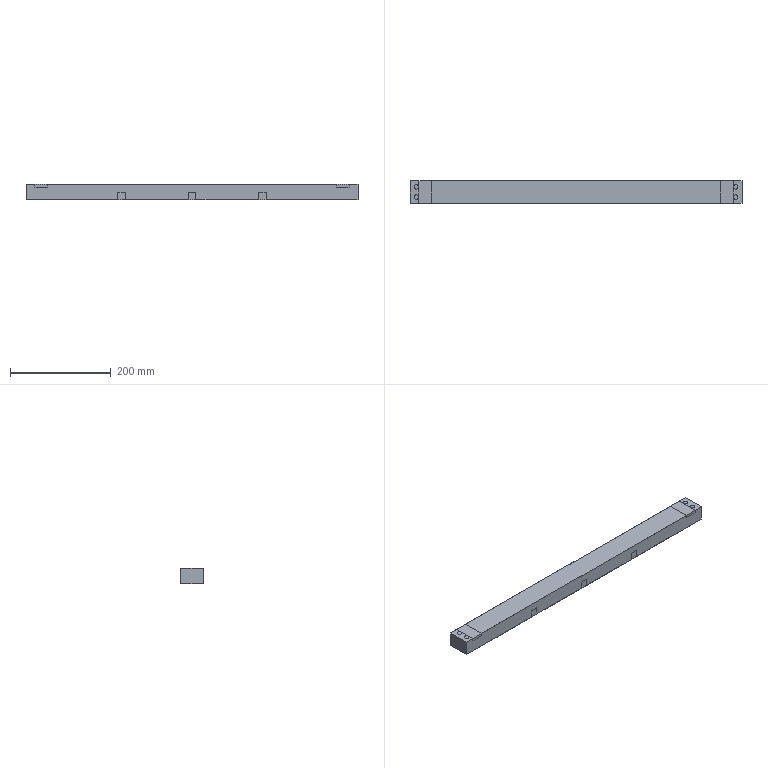NC program | NX | posted with a generic post | part box 659.9 x 45 x 30 mm
Whole program:
N10 G17 G21 G94 G90
(FLOOR_WALL_1 , TOOL : D63)
N12 T01 M6
N14 G54
N16 G17 G0 G90 X-364.45 Y0. S6500 M3
N18 G43 Z30. H1
N20 Z3.
N22 G94 G1 Z0. F1250.
N24 X-361.45
N26 X361.45
N28 X364.45
N30 Z3.
N32 G0 Z30.
N34 M5
N36 M2